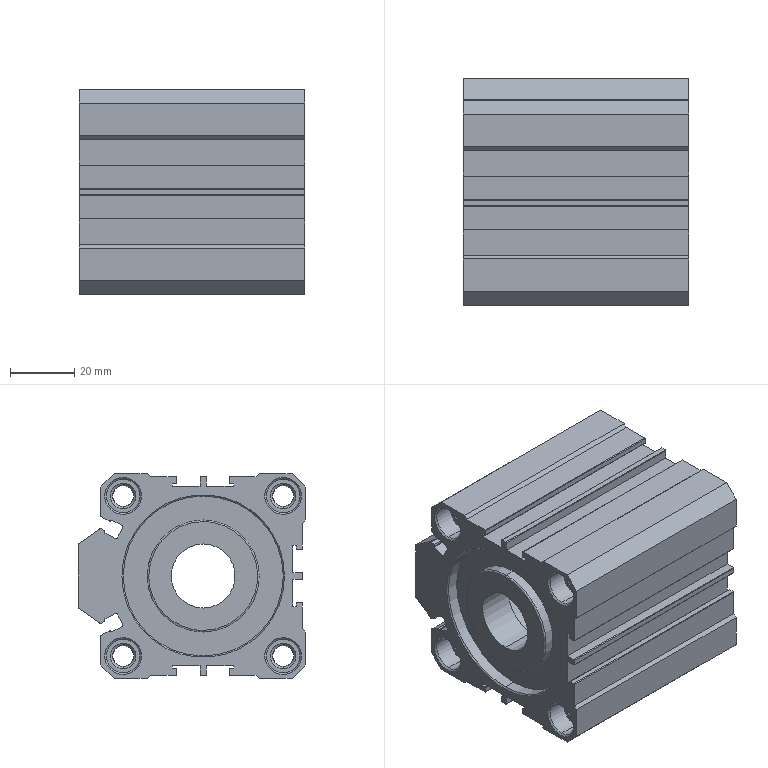Part | SolidWorks | features BaseBody 1 | 1 solid | 264 faces | box 70.5 x 71 x 64 mm | volume 156826 mm3 | cylinder 108 | plane 96 | cone 56 | spline 4 | commonest cylinder face diameters 0.4 x35 6.647 x16 10.5 x16 0.8 x15 6.5 x8 50 x6